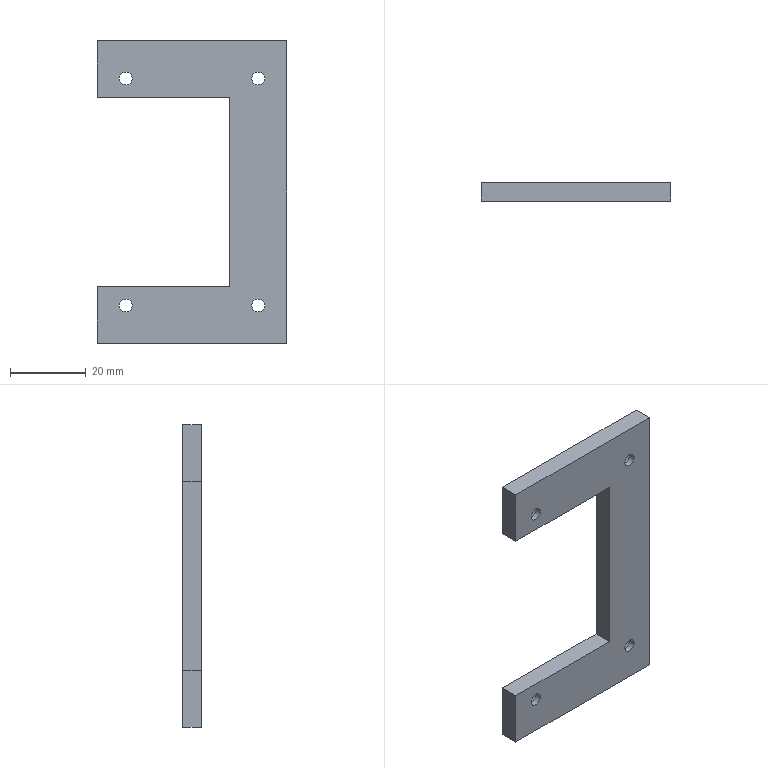Part | NX | 1 solid | 22 faces | box 50 x 5 x 80 mm | volume 10741 mm3 | plane 14 | cylinder 8 | commonest cylinder face diameters 3.4 x4 6.5 x4
STEP:
#1=CARTESIAN_POINT('',(-25.,0.,-40.));
#2=VERTEX_POINT('',#1);
#3=CARTESIAN_POINT('',(-25.,0.,-25.));
#4=VERTEX_POINT('',#3);
#5=CARTESIAN_POINT('',(-25.,0.,40.));
#6=DIRECTION('',(0.,0.,1.));
#7=VECTOR('',#6,1000.);
#8=LINE('',#5,#7);
#9=EDGE_CURVE('',#2,#4,#8,.T.);
#10=ORIENTED_EDGE('',*,*,#9,.T.);
#11=CARTESIAN_POINT('',(-25.,5.,-25.));
#12=VERTEX_POINT('',#11);
#13=CARTESIAN_POINT('',(-25.,0.,-25.));
#14=DIRECTION('',(0.,1.,0.));
#15=VECTOR('',#14,1000.);
#16=LINE('',#13,#15);
#17=EDGE_CURVE('',#4,#12,#16,.T.);
#18=ORIENTED_EDGE('',*,*,#17,.T.);
#19=CARTESIAN_POINT('',(-25.,5.,-40.));
#20=VERTEX_POINT('',#19);
#21=CARTESIAN_POINT('',(-25.,5.,40.));
#22=DIRECTION('',(0.,0.,1.));
#23=VECTOR('',#22,1000.);
#24=LINE('',#21,#23);
#25=EDGE_CURVE('',#20,#12,#24,.T.);
#26=ORIENTED_EDGE('',*,*,#25,.F.);
#27=CARTESIAN_POINT('',(-25.,5.,-40.));
#28=DIRECTION('',(0.,-1.,0.));
#29=VECTOR('',#28,1000.);
#30=LINE('',#27,#29);
#31=EDGE_CURVE('',#20,#2,#30,.T.);
#32=ORIENTED_EDGE('',*,*,#31,.T.);
#33=EDGE_LOOP('',(#10,#18,#26,#32));
#34=FACE_BOUND('',#33,.T.);
#35=CARTESIAN_POINT('',(-25.,5.,40.));
#36=DIRECTION('',(1.,0.,0.));
#37=DIRECTION('',(0.,0.,-1.));
#38=AXIS2_PLACEMENT_3D('',#35,#36,#37);
#39=PLANE('',#38);
#40=ADVANCED_FACE('',(#34),#39,.F.);
#41=CARTESIAN_POINT('',(25.,0.,40.));
#42=VERTEX_POINT('',#41);
#43=CARTESIAN_POINT('',(25.,0.,-40.));
#44=VERTEX_POINT('',#43);
#45=CARTESIAN_POINT('',(25.,0.,40.));
#46=DIRECTION('',(0.,0.,-1.));
#47=VECTOR('',#46,1000.);
#48=LINE('',#45,#47);
#49=EDGE_CURVE('',#42,#44,#48,.T.);
#50=ORIENTED_EDGE('',*,*,#49,.T.);
#51=CARTESIAN_POINT('',(25.,5.,-40.));
#52=VERTEX_POINT('',#51);
#53=CARTESIAN_POINT('',(25.,5.,-40.));
#54=DIRECTION('',(0.,-1.,0.));
#55=VECTOR('',#54,1000.);
#56=LINE('',#53,#55);
#57=EDGE_CURVE('',#52,#44,#56,.T.);
#58=ORIENTED_EDGE('',*,*,#57,.F.);
#59=CARTESIAN_POINT('',(25.,5.,40.));
#60=VERTEX_POINT('',#59);
#61=CARTESIAN_POINT('',(25.,5.,40.));
#62=DIRECTION('',(0.,0.,-1.));
#63=VECTOR('',#62,1000.);
#64=LINE('',#61,#63);
#65=EDGE_CURVE('',#60,#52,#64,.T.);
#66=ORIENTED_EDGE('',*,*,#65,.F.);
#67=CARTESIAN_POINT('',(25.,5.,40.));
#68=DIRECTION('',(0.,-1.,0.));
#69=VECTOR('',#68,1000.);
#70=LINE('',#67,#69);
#71=EDGE_CURVE('',#60,#42,#70,.T.);
#72=ORIENTED_EDGE('',*,*,#71,.T.);
#73=EDGE_LOOP('',(#50,#58,#66,#72));
#74=FACE_BOUND('',#73,.T.);
#75=CARTESIAN_POINT('',(25.,5.,40.));
#76=DIRECTION('',(-1.,0.,0.));
#77=DIRECTION('',(0.,0.,1.));
#78=AXIS2_PLACEMENT_3D('',#75,#76,#77);
#79=PLANE('',#78);
#80=ADVANCED_FACE('',(#74),#79,.F.);
#81=CARTESIAN_POINT('',(-25.,0.,-40.));
#82=DIRECTION('',(-1.,0.,0.));
#83=VECTOR('',#82,1000.);
#84=LINE('',#81,#83);
#85=EDGE_CURVE('',#44,#2,#84,.T.);
#86=ORIENTED_EDGE('',*,*,#85,.T.);
#87=ORIENTED_EDGE('',*,*,#31,.F.);
#88=CARTESIAN_POINT('',(-25.,5.,-40.));
#89=DIRECTION('',(-1.,0.,0.));
#90=VECTOR('',#89,1000.);
#91=LINE('',#88,#90);
#92=EDGE_CURVE('',#52,#20,#91,.T.);
#93=ORIENTED_EDGE('',*,*,#92,.F.);
#94=ORIENTED_EDGE('',*,*,#57,.T.);
#95=EDGE_LOOP('',(#86,#87,#93,#94));
#96=FACE_BOUND('',#95,.T.);
#97=CARTESIAN_POINT('',(-25.,5.,-40.));
#98=DIRECTION('',(0.,0.,1.));
#99=DIRECTION('',(1.,0.,0.));
#100=AXIS2_PLACEMENT_3D('',#97,#98,#99);
#101=PLANE('',#100);
#102=ADVANCED_FACE('',(#96),#101,.F.);
#103=CARTESIAN_POINT('',(-25.,5.,25.));
#104=VERTEX_POINT('',#103);
#105=CARTESIAN_POINT('',(-25.,5.,40.));
#106=VERTEX_POINT('',#105);
#107=CARTESIAN_POINT('',(-25.,5.,40.));
#108=DIRECTION('',(0.,0.,1.));
#109=VECTOR('',#108,1000.);
#110=LINE('',#107,#109);
#111=EDGE_CURVE('',#104,#106,#110,.T.);
#112=ORIENTED_EDGE('',*,*,#111,.F.);
#113=CARTESIAN_POINT('',(-25.,0.,25.));
#114=VERTEX_POINT('',#113);
#115=CARTESIAN_POINT('',(-25.,0.,25.));
#116=DIRECTION('',(0.,1.,0.));
#117=VECTOR('',#116,1000.);
#118=LINE('',#115,#117);
#119=EDGE_CURVE('',#114,#104,#118,.T.);
#120=ORIENTED_EDGE('',*,*,#119,.F.);
#121=CARTESIAN_POINT('',(-25.,0.,40.));
#122=VERTEX_POINT('',#121);
#123=CARTESIAN_POINT('',(-25.,0.,40.));
#124=DIRECTION('',(0.,0.,1.));
#125=VECTOR('',#124,1000.);
#126=LINE('',#123,#125);
#127=EDGE_CURVE('',#114,#122,#126,.T.);
#128=ORIENTED_EDGE('',*,*,#127,.T.);
#129=CARTESIAN_POINT('',(-25.,5.,40.));
#130=DIRECTION('',(0.,-1.,0.));
#131=VECTOR('',#130,1000.);
#132=LINE('',#129,#131);
#133=EDGE_CURVE('',#106,#122,#132,.T.);
#134=ORIENTED_EDGE('',*,*,#133,.F.);
#135=EDGE_LOOP('',(#112,#120,#128,#134));
#136=FACE_BOUND('',#135,.T.);
#137=CARTESIAN_POINT('',(-25.,5.,40.));
#138=DIRECTION('',(1.,0.,0.));
#139=DIRECTION('',(0.,0.,-1.));
#140=AXIS2_PLACEMENT_3D('',#137,#138,#139);
#141=PLANE('',#140);
#142=ADVANCED_FACE('',(#136),#141,.F.);
#143=CARTESIAN_POINT('',(-25.,0.,40.));
#144=DIRECTION('',(1.,0.,0.));
#145=VECTOR('',#144,1000.);
#146=LINE('',#143,#145);
#147=EDGE_CURVE('',#122,#42,#146,.T.);
#148=ORIENTED_EDGE('',*,*,#147,.T.);
#149=ORIENTED_EDGE('',*,*,#71,.F.);
#150=CARTESIAN_POINT('',(-25.,5.,40.));
#151=DIRECTION('',(1.,0.,0.));
#152=VECTOR('',#151,1000.);
#153=LINE('',#150,#152);
#154=EDGE_CURVE('',#106,#60,#153,.T.);
#155=ORIENTED_EDGE('',*,*,#154,.F.);
#156=ORIENTED_EDGE('',*,*,#133,.T.);
#157=EDGE_LOOP('',(#148,#149,#155,#156));
#158=FACE_BOUND('',#157,.T.);
#159=CARTESIAN_POINT('',(-25.,5.,40.));
#160=DIRECTION('',(0.,0.,-1.));
#161=DIRECTION('',(-1.,0.,0.));
#162=AXIS2_PLACEMENT_3D('',#159,#160,#161);
#163=PLANE('',#162);
#164=ADVANCED_FACE('',(#158),#163,.F.);
#165=CARTESIAN_POINT('',(-17.5,5.,-26.75));
#166=VERTEX_POINT('',#165);
#167=CARTESIAN_POINT('',(-17.5,5.,-30.));
#168=DIRECTION('',(0.,1.,0.));
#169=DIRECTION('',(0.,0.,1.));
#170=AXIS2_PLACEMENT_3D('',#167,#168,#169);
#171=CIRCLE('',#170,3.25);
#172=EDGE_CURVE('',#166,#166,#171,.T.);
#173=ORIENTED_EDGE('',*,*,#172,.F.);
#174=EDGE_LOOP('',(#173));
#175=FACE_BOUND('',#174,.T.);
#176=CARTESIAN_POINT('',(17.5,5.,-26.75));
#177=VERTEX_POINT('',#176);
#178=CARTESIAN_POINT('',(17.5,5.,-30.));
#179=DIRECTION('',(0.,1.,0.));
#180=DIRECTION('',(0.,0.,1.));
#181=AXIS2_PLACEMENT_3D('',#178,#179,#180);
#182=CIRCLE('',#181,3.25);
#183=EDGE_CURVE('',#177,#177,#182,.T.);
#184=ORIENTED_EDGE('',*,*,#183,.F.);
#185=EDGE_LOOP('',(#184));
#186=FACE_BOUND('',#185,.T.);
#187=CARTESIAN_POINT('',(17.5,5.,33.25));
#188=VERTEX_POINT('',#187);
#189=CARTESIAN_POINT('',(17.5,5.,30.));
#190=DIRECTION('',(0.,1.,0.));
#191=DIRECTION('',(0.,0.,1.));
#192=AXIS2_PLACEMENT_3D('',#189,#190,#191);
#193=CIRCLE('',#192,3.25);
#194=EDGE_CURVE('',#188,#188,#193,.T.);
#195=ORIENTED_EDGE('',*,*,#194,.F.);
#196=EDGE_LOOP('',(#195));
#197=FACE_BOUND('',#196,.T.);
#198=CARTESIAN_POINT('',(-17.5,5.,33.25));
#199=VERTEX_POINT('',#198);
#200=CARTESIAN_POINT('',(-17.5,5.,30.));
#201=DIRECTION('',(0.,1.,0.));
#202=DIRECTION('',(0.,0.,1.));
#203=AXIS2_PLACEMENT_3D('',#200,#201,#202);
#204=CIRCLE('',#203,3.25);
#205=EDGE_CURVE('',#199,#199,#204,.T.);
#206=ORIENTED_EDGE('',*,*,#205,.F.);
#207=EDGE_LOOP('',(#206));
#208=FACE_BOUND('',#207,.T.);
#209=ORIENTED_EDGE('',*,*,#25,.T.);
#210=CARTESIAN_POINT('',(10.,5.,-25.));
#211=VERTEX_POINT('',#210);
#212=CARTESIAN_POINT('',(10.,5.,-25.));
#213=DIRECTION('',(-1.,0.,0.));
#214=VECTOR('',#213,1000.);
#215=LINE('',#212,#214);
#216=EDGE_CURVE('',#211,#12,#215,.T.);
#217=ORIENTED_EDGE('',*,*,#216,.F.);
#218=CARTESIAN_POINT('',(10.,5.,25.));
#219=VERTEX_POINT('',#218);
#220=CARTESIAN_POINT('',(10.,5.,25.));
#221=DIRECTION('',(0.,0.,-1.));
#222=VECTOR('',#221,1000.);
#223=LINE('',#220,#222);
#224=EDGE_CURVE('',#219,#211,#223,.T.);
#225=ORIENTED_EDGE('',*,*,#224,.F.);
#226=CARTESIAN_POINT('',(10.,5.,25.));
#227=DIRECTION('',(1.,0.,0.));
#228=VECTOR('',#227,1000.);
#229=LINE('',#226,#228);
#230=EDGE_CURVE('',#104,#219,#229,.T.);
#231=ORIENTED_EDGE('',*,*,#230,.F.);
#232=ORIENTED_EDGE('',*,*,#111,.T.);
#233=ORIENTED_EDGE('',*,*,#154,.T.);
#234=ORIENTED_EDGE('',*,*,#65,.T.);
#235=ORIENTED_EDGE('',*,*,#92,.T.);
#236=EDGE_LOOP('',(#209,#217,#225,#231,#232,#233,#234,#235));
#237=FACE_BOUND('',#236,.T.);
#238=CARTESIAN_POINT('',(0.,5.,0.));
#239=DIRECTION('',(0.,-1.,0.));
#240=DIRECTION('',(0.,0.,-1.));
#241=AXIS2_PLACEMENT_3D('',#238,#239,#240);
#242=PLANE('',#241);
#243=ADVANCED_FACE('',(#175,#186,#197,#208,#237),#242,.F.);
#244=CARTESIAN_POINT('',(10.,0.,-25.));
#245=VERTEX_POINT('',#244);
#246=CARTESIAN_POINT('',(10.,0.,-25.));
#247=DIRECTION('',(-1.,0.,0.));
#248=VECTOR('',#247,1000.);
#249=LINE('',#246,#248);
#250=EDGE_CURVE('',#245,#4,#249,.T.);
#251=ORIENTED_EDGE('',*,*,#250,.T.);
#252=ORIENTED_EDGE('',*,*,#9,.F.);
#253=ORIENTED_EDGE('',*,*,#85,.F.);
#254=ORIENTED_EDGE('',*,*,#49,.F.);
#255=ORIENTED_EDGE('',*,*,#147,.F.);
#256=ORIENTED_EDGE('',*,*,#127,.F.);
#257=CARTESIAN_POINT('',(10.,0.,25.));
#258=VERTEX_POINT('',#257);
#259=CARTESIAN_POINT('',(10.,0.,25.));
#260=DIRECTION('',(1.,0.,0.));
#261=VECTOR('',#260,1000.);
#262=LINE('',#259,#261);
#263=EDGE_CURVE('',#114,#258,#262,.T.);
#264=ORIENTED_EDGE('',*,*,#263,.T.);
#265=CARTESIAN_POINT('',(10.,0.,25.));
#266=DIRECTION('',(0.,0.,-1.));
#267=VECTOR('',#266,1000.);
#268=LINE('',#265,#267);
#269=EDGE_CURVE('',#258,#245,#268,.T.);
#270=ORIENTED_EDGE('',*,*,#269,.T.);
#271=EDGE_LOOP('',(#251,#252,#253,#254,#255,#256,#264,#270));
#272=FACE_BOUND('',#271,.T.);
#273=CARTESIAN_POINT('',(-17.5,0.,-28.3));
#274=VERTEX_POINT('',#273);
#275=CARTESIAN_POINT('',(-17.5,0.,-30.));
#276=DIRECTION('',(0.,1.,0.));
#277=DIRECTION('',(0.,0.,1.));
#278=AXIS2_PLACEMENT_3D('',#275,#276,#277);
#279=CIRCLE('',#278,1.7);
#280=EDGE_CURVE('',#274,#274,#279,.T.);
#281=ORIENTED_EDGE('',*,*,#280,.T.);
#282=EDGE_LOOP('',(#281));
#283=FACE_BOUND('',#282,.T.);
#284=CARTESIAN_POINT('',(17.5,0.,-28.3));
#285=VERTEX_POINT('',#284);
#286=CARTESIAN_POINT('',(17.5,0.,-30.));
#287=DIRECTION('',(0.,1.,0.));
#288=DIRECTION('',(0.,0.,1.));
#289=AXIS2_PLACEMENT_3D('',#286,#287,#288);
#290=CIRCLE('',#289,1.7);
#291=EDGE_CURVE('',#285,#285,#290,.T.);
#292=ORIENTED_EDGE('',*,*,#291,.T.);
#293=EDGE_LOOP('',(#292));
#294=FACE_BOUND('',#293,.T.);
#295=CARTESIAN_POINT('',(17.5,0.,31.7));
#296=VERTEX_POINT('',#295);
#297=CARTESIAN_POINT('',(17.5,0.,30.));
#298=DIRECTION('',(0.,1.,0.));
#299=DIRECTION('',(0.,0.,1.));
#300=AXIS2_PLACEMENT_3D('',#297,#298,#299);
#301=CIRCLE('',#300,1.7);
#302=EDGE_CURVE('',#296,#296,#301,.T.);
#303=ORIENTED_EDGE('',*,*,#302,.T.);
#304=EDGE_LOOP('',(#303));
#305=FACE_BOUND('',#304,.T.);
#306=CARTESIAN_POINT('',(-17.5,0.,31.7));
#307=VERTEX_POINT('',#306);
#308=CARTESIAN_POINT('',(-17.5,0.,30.));
#309=DIRECTION('',(0.,1.,0.));
#310=DIRECTION('',(0.,0.,1.));
#311=AXIS2_PLACEMENT_3D('',#308,#309,#310);
#312=CIRCLE('',#311,1.7);
#313=EDGE_CURVE('',#307,#307,#312,.T.);
#314=ORIENTED_EDGE('',*,*,#313,.T.);
#315=EDGE_LOOP('',(#314));
#316=FACE_BOUND('',#315,.T.);
#317=CARTESIAN_POINT('',(0.,0.,0.));
#318=DIRECTION('',(0.,-1.,0.));
#319=DIRECTION('',(0.,0.,-1.));
#320=AXIS2_PLACEMENT_3D('',#317,#318,#319);
#321=PLANE('',#320);
#322=ADVANCED_FACE('',(#272,#283,#294,#305,#316),#321,.T.);
#323=ORIENTED_EDGE('',*,*,#313,.F.);
#324=EDGE_LOOP('',(#323));
#325=FACE_BOUND('',#324,.T.);
#326=CARTESIAN_POINT('',(-17.5,1.6,31.7));
#327=VERTEX_POINT('',#326);
#328=CARTESIAN_POINT('',(-17.5,1.6,30.));
#329=DIRECTION('',(0.,1.,0.));
#330=DIRECTION('',(0.,0.,1.));
#331=AXIS2_PLACEMENT_3D('',#328,#329,#330);
#332=CIRCLE('',#331,1.7);
#333=EDGE_CURVE('',#327,#327,#332,.T.);
#334=ORIENTED_EDGE('',*,*,#333,.T.);
#335=EDGE_LOOP('',(#334));
#336=FACE_BOUND('',#335,.T.);
#337=CARTESIAN_POINT('',(-17.5,5.,30.));
#338=DIRECTION('',(0.,1.,0.));
#339=DIRECTION('',(0.,0.,1.));
#340=AXIS2_PLACEMENT_3D('',#337,#338,#339);
#341=CYLINDRICAL_SURFACE('',#340,1.7);
#342=ADVANCED_FACE('',(#325,#336),#341,.F.);
#343=ORIENTED_EDGE('',*,*,#333,.F.);
#344=EDGE_LOOP('',(#343));
#345=FACE_BOUND('',#344,.T.);
#346=CARTESIAN_POINT('',(-17.5,1.6,33.25));
#347=VERTEX_POINT('',#346);
#348=CARTESIAN_POINT('',(-17.5,1.6,30.));
#349=DIRECTION('',(0.,1.,0.));
#350=DIRECTION('',(0.,0.,1.));
#351=AXIS2_PLACEMENT_3D('',#348,#349,#350);
#352=CIRCLE('',#351,3.25);
#353=EDGE_CURVE('',#347,#347,#352,.T.);
#354=ORIENTED_EDGE('',*,*,#353,.T.);
#355=EDGE_LOOP('',(#354));
#356=FACE_BOUND('',#355,.T.);
#357=CARTESIAN_POINT('',(-15.8,1.6,30.));
#358=DIRECTION('',(0.,-1.,0.));
#359=DIRECTION('',(0.,0.,-1.));
#360=AXIS2_PLACEMENT_3D('',#357,#358,#359);
#361=PLANE('',#360);
#362=ADVANCED_FACE('',(#345,#356),#361,.F.);
#363=ORIENTED_EDGE('',*,*,#353,.F.);
#364=EDGE_LOOP('',(#363));
#365=FACE_BOUND('',#364,.T.);
#366=ORIENTED_EDGE('',*,*,#205,.T.);
#367=EDGE_LOOP('',(#366));
#368=FACE_BOUND('',#367,.T.);
#369=CARTESIAN_POINT('',(-17.5,5.,30.));
#370=DIRECTION('',(0.,1.,0.));
#371=DIRECTION('',(0.,0.,1.));
#372=AXIS2_PLACEMENT_3D('',#369,#370,#371);
#373=CYLINDRICAL_SURFACE('',#372,3.25);
#374=ADVANCED_FACE('',(#365,#368),#373,.F.);
#375=ORIENTED_EDGE('',*,*,#302,.F.);
#376=EDGE_LOOP('',(#375));
#377=FACE_BOUND('',#376,.T.);
#378=CARTESIAN_POINT('',(17.5,1.6,31.7));
#379=VERTEX_POINT('',#378);
#380=CARTESIAN_POINT('',(17.5,1.6,30.));
#381=DIRECTION('',(0.,1.,0.));
#382=DIRECTION('',(0.,0.,1.));
#383=AXIS2_PLACEMENT_3D('',#380,#381,#382);
#384=CIRCLE('',#383,1.7);
#385=EDGE_CURVE('',#379,#379,#384,.T.);
#386=ORIENTED_EDGE('',*,*,#385,.T.);
#387=EDGE_LOOP('',(#386));
#388=FACE_BOUND('',#387,.T.);
#389=CARTESIAN_POINT('',(17.5,5.,30.));
#390=DIRECTION('',(0.,1.,0.));
#391=DIRECTION('',(0.,0.,1.));
#392=AXIS2_PLACEMENT_3D('',#389,#390,#391);
#393=CYLINDRICAL_SURFACE('',#392,1.7);
#394=ADVANCED_FACE('',(#377,#388),#393,.F.);
#395=ORIENTED_EDGE('',*,*,#385,.F.);
#396=EDGE_LOOP('',(#395));
#397=FACE_BOUND('',#396,.T.);
#398=CARTESIAN_POINT('',(17.5,1.6,33.25));
#399=VERTEX_POINT('',#398);
#400=CARTESIAN_POINT('',(17.5,1.6,30.));
#401=DIRECTION('',(0.,1.,0.));
#402=DIRECTION('',(0.,0.,1.));
#403=AXIS2_PLACEMENT_3D('',#400,#401,#402);
#404=CIRCLE('',#403,3.25);
#405=EDGE_CURVE('',#399,#399,#404,.T.);
#406=ORIENTED_EDGE('',*,*,#405,.T.);
#407=EDGE_LOOP('',(#406));
#408=FACE_BOUND('',#407,.T.);
#409=CARTESIAN_POINT('',(19.2,1.6,30.));
#410=DIRECTION('',(0.,-1.,0.));
#411=DIRECTION('',(0.,0.,-1.));
#412=AXIS2_PLACEMENT_3D('',#409,#410,#411);
#413=PLANE('',#412);
#414=ADVANCED_FACE('',(#397,#408),#413,.F.);
#415=ORIENTED_EDGE('',*,*,#405,.F.);
#416=EDGE_LOOP('',(#415));
#417=FACE_BOUND('',#416,.T.);
#418=ORIENTED_EDGE('',*,*,#194,.T.);
#419=EDGE_LOOP('',(#418));
#420=FACE_BOUND('',#419,.T.);
#421=CARTESIAN_POINT('',(17.5,5.,30.));
#422=DIRECTION('',(0.,1.,0.));
#423=DIRECTION('',(0.,0.,1.));
#424=AXIS2_PLACEMENT_3D('',#421,#422,#423);
#425=CYLINDRICAL_SURFACE('',#424,3.25);
#426=ADVANCED_FACE('',(#417,#420),#425,.F.);
#427=ORIENTED_EDGE('',*,*,#291,.F.);
#428=EDGE_LOOP('',(#427));
#429=FACE_BOUND('',#428,.T.);
#430=CARTESIAN_POINT('',(17.5,1.6,-28.3));
#431=VERTEX_POINT('',#430);
#432=CARTESIAN_POINT('',(17.5,1.6,-30.));
#433=DIRECTION('',(0.,1.,0.));
#434=DIRECTION('',(0.,0.,1.));
#435=AXIS2_PLACEMENT_3D('',#432,#433,#434);
#436=CIRCLE('',#435,1.7);
#437=EDGE_CURVE('',#431,#431,#436,.T.);
#438=ORIENTED_EDGE('',*,*,#437,.T.);
#439=EDGE_LOOP('',(#438));
#440=FACE_BOUND('',#439,.T.);
#441=CARTESIAN_POINT('',(17.5,5.,-30.));
#442=DIRECTION('',(0.,1.,0.));
#443=DIRECTION('',(0.,0.,1.));
#444=AXIS2_PLACEMENT_3D('',#441,#442,#443);
#445=CYLINDRICAL_SURFACE('',#444,1.7);
#446=ADVANCED_FACE('',(#429,#440),#445,.F.);
#447=ORIENTED_EDGE('',*,*,#437,.F.);
#448=EDGE_LOOP('',(#447));
#449=FACE_BOUND('',#448,.T.);
#450=CARTESIAN_POINT('',(17.5,1.6,-26.75));
#451=VERTEX_POINT('',#450);
#452=CARTESIAN_POINT('',(17.5,1.6,-30.));
#453=DIRECTION('',(0.,1.,0.));
#454=DIRECTION('',(0.,0.,1.));
#455=AXIS2_PLACEMENT_3D('',#452,#453,#454);
#456=CIRCLE('',#455,3.25);
#457=EDGE_CURVE('',#451,#451,#456,.T.);
#458=ORIENTED_EDGE('',*,*,#457,.T.);
#459=EDGE_LOOP('',(#458));
#460=FACE_BOUND('',#459,.T.);
#461=CARTESIAN_POINT('',(19.2,1.6,-30.));
#462=DIRECTION('',(0.,-1.,0.));
#463=DIRECTION('',(0.,0.,-1.));
#464=AXIS2_PLACEMENT_3D('',#461,#462,#463);
#465=PLANE('',#464);
#466=ADVANCED_FACE('',(#449,#460),#465,.F.);
#467=ORIENTED_EDGE('',*,*,#457,.F.);
#468=EDGE_LOOP('',(#467));
#469=FACE_BOUND('',#468,.T.);
#470=ORIENTED_EDGE('',*,*,#183,.T.);
#471=EDGE_LOOP('',(#470));
#472=FACE_BOUND('',#471,.T.);
#473=CARTESIAN_POINT('',(17.5,5.,-30.));
#474=DIRECTION('',(0.,1.,0.));
#475=DIRECTION('',(0.,0.,1.));
#476=AXIS2_PLACEMENT_3D('',#473,#474,#475);
#477=CYLINDRICAL_SURFACE('',#476,3.25);
#478=ADVANCED_FACE('',(#469,#472),#477,.F.);
#479=ORIENTED_EDGE('',*,*,#280,.F.);
#480=EDGE_LOOP('',(#479));
#481=FACE_BOUND('',#480,.T.);
#482=CARTESIAN_POINT('',(-17.5,1.6,-28.3));
#483=VERTEX_POINT('',#482);
#484=CARTESIAN_POINT('',(-17.5,1.6,-30.));
#485=DIRECTION('',(0.,1.,0.));
#486=DIRECTION('',(0.,0.,1.));
#487=AXIS2_PLACEMENT_3D('',#484,#485,#486);
#488=CIRCLE('',#487,1.7);
#489=EDGE_CURVE('',#483,#483,#488,.T.);
#490=ORIENTED_EDGE('',*,*,#489,.T.);
#491=EDGE_LOOP('',(#490));
#492=FACE_BOUND('',#491,.T.);
#493=CARTESIAN_POINT('',(-17.5,5.,-30.));
#494=DIRECTION('',(0.,1.,0.));
#495=DIRECTION('',(0.,0.,1.));
#496=AXIS2_PLACEMENT_3D('',#493,#494,#495);
#497=CYLINDRICAL_SURFACE('',#496,1.7);
#498=ADVANCED_FACE('',(#481,#492),#497,.F.);
#499=ORIENTED_EDGE('',*,*,#489,.F.);
#500=EDGE_LOOP('',(#499));
#501=FACE_BOUND('',#500,.T.);
#502=CARTESIAN_POINT('',(-17.5,1.6,-26.75));
#503=VERTEX_POINT('',#502);
#504=CARTESIAN_POINT('',(-17.5,1.6,-30.));
#505=DIRECTION('',(0.,1.,0.));
#506=DIRECTION('',(0.,0.,1.));
#507=AXIS2_PLACEMENT_3D('',#504,#505,#506);
#508=CIRCLE('',#507,3.25);
#509=EDGE_CURVE('',#503,#503,#508,.T.);
#510=ORIENTED_EDGE('',*,*,#509,.T.);
#511=EDGE_LOOP('',(#510));
#512=FACE_BOUND('',#511,.T.);
#513=CARTESIAN_POINT('',(-15.8,1.6,-30.));
#514=DIRECTION('',(0.,-1.,0.));
#515=DIRECTION('',(0.,0.,-1.));
#516=AXIS2_PLACEMENT_3D('',#513,#514,#515);
#517=PLANE('',#516);
#518=ADVANCED_FACE('',(#501,#512),#517,.F.);
#519=ORIENTED_EDGE('',*,*,#509,.F.);
#520=EDGE_LOOP('',(#519));
#521=FACE_BOUND('',#520,.T.);
#522=ORIENTED_EDGE('',*,*,#172,.T.);
#523=EDGE_LOOP('',(#522));
#524=FACE_BOUND('',#523,.T.);
#525=CARTESIAN_POINT('',(-17.5,5.,-30.));
#526=DIRECTION('',(0.,1.,0.));
#527=DIRECTION('',(0.,0.,1.));
#528=AXIS2_PLACEMENT_3D('',#525,#526,#527);
#529=CYLINDRICAL_SURFACE('',#528,3.25);
#530=ADVANCED_FACE('',(#521,#524),#529,.F.);
#531=ORIENTED_EDGE('',*,*,#216,.T.);
#532=ORIENTED_EDGE('',*,*,#17,.F.);
#533=ORIENTED_EDGE('',*,*,#250,.F.);
#534=CARTESIAN_POINT('',(10.,0.,-25.));
#535=DIRECTION('',(0.,1.,0.));
#536=VECTOR('',#535,1000.);
#537=LINE('',#534,#536);
#538=EDGE_CURVE('',#245,#211,#537,.T.);
#539=ORIENTED_EDGE('',*,*,#538,.T.);
#540=EDGE_LOOP('',(#531,#532,#533,#539));
#541=FACE_BOUND('',#540,.T.);
#542=CARTESIAN_POINT('',(10.,0.,-25.));
#543=DIRECTION('',(0.,0.,-1.));
#544=DIRECTION('',(-1.,0.,0.));
#545=AXIS2_PLACEMENT_3D('',#542,#543,#544);
#546=PLANE('',#545);
#547=ADVANCED_FACE('',(#541),#546,.F.);
#548=ORIENTED_EDGE('',*,*,#224,.T.);
#549=ORIENTED_EDGE('',*,*,#538,.F.);
#550=ORIENTED_EDGE('',*,*,#269,.F.);
#551=CARTESIAN_POINT('',(10.,0.,25.));
#552=DIRECTION('',(0.,1.,0.));
#553=VECTOR('',#552,1000.);
#554=LINE('',#551,#553);
#555=EDGE_CURVE('',#258,#219,#554,.T.);
#556=ORIENTED_EDGE('',*,*,#555,.T.);
#557=EDGE_LOOP('',(#548,#549,#550,#556));
#558=FACE_BOUND('',#557,.T.);
#559=CARTESIAN_POINT('',(10.,0.,25.));
#560=DIRECTION('',(1.,0.,0.));
#561=DIRECTION('',(0.,0.,-1.));
#562=AXIS2_PLACEMENT_3D('',#559,#560,#561);
#563=PLANE('',#562);
#564=ADVANCED_FACE('',(#558),#563,.F.);
#565=ORIENTED_EDGE('',*,*,#230,.T.);
#566=ORIENTED_EDGE('',*,*,#555,.F.);
#567=ORIENTED_EDGE('',*,*,#263,.F.);
#568=ORIENTED_EDGE('',*,*,#119,.T.);
#569=EDGE_LOOP('',(#565,#566,#567,#568));
#570=FACE_BOUND('',#569,.T.);
#571=CARTESIAN_POINT('',(10.,0.,25.));
#572=DIRECTION('',(0.,0.,1.));
#573=DIRECTION('',(1.,0.,0.));
#574=AXIS2_PLACEMENT_3D('',#571,#572,#573);
#575=PLANE('',#574);
#576=ADVANCED_FACE('',(#570),#575,.F.);
#577=CLOSED_SHELL('',(#40,#80,#102,#142,#164,#243,#322,#342,#362,#374,#394,#414,#426,#446,#466,#478,#498,#518,#530,#547,#564,#576));
#578=MANIFOLD_SOLID_BREP('',#577);
#579=(LENGTH_UNIT()NAMED_UNIT(*)SI_UNIT(.MILLI.,.METRE.));
#580=UNCERTAINTY_MEASURE_WITH_UNIT(LENGTH_MEASURE(0.00001),#579,'','');
#581=(NAMED_UNIT(*)PLANE_ANGLE_UNIT()SI_UNIT($,.RADIAN.));
#582=(NAMED_UNIT(*)SI_UNIT($,.STERADIAN.)SOLID_ANGLE_UNIT());
#583=(GEOMETRIC_REPRESENTATION_CONTEXT(3)GLOBAL_UNCERTAINTY_ASSIGNED_CONTEXT((#580))GLOBAL_UNIT_ASSIGNED_CONTEXT((#579,#581,#582))REPRESENTATION_CONTEXT('',''));
#584=ADVANCED_BREP_SHAPE_REPRESENTATION('',(#578),#583);